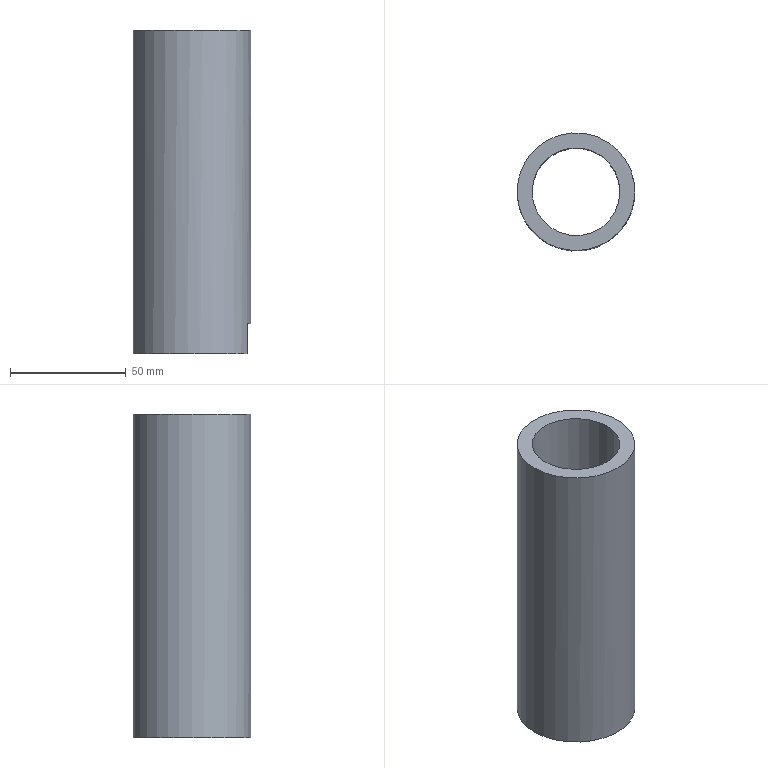Part | NX | features solid 2 | 1 solid | 7 faces | box 51 x 51 x 140 mm | volume 125652 mm3 | plane 5 | cylinder 2 | commonest cylinder face diameters 38 x1 51 x1
STEP:
#1=CARTESIAN_POINT('',(329.506,538.888,40.));
#2=VERTEX_POINT('',#1);
#3=CARTESIAN_POINT('',(348.506,538.888,40.));
#4=DIRECTION('',(0.,0.,1.));
#5=DIRECTION('',(-1.,0.,0.));
#6=AXIS2_PLACEMENT_3D('',#3,#4,#5);
#7=CIRCLE('',#6,19.);
#8=EDGE_CURVE('',#2,#2,#7,.F.);
#9=ORIENTED_EDGE('',*,*,#8,.T.);
#10=EDGE_LOOP('',(#9));
#11=FACE_BOUND('',#10,.T.);
#12=CARTESIAN_POINT('',(323.006,538.888,40.));
#13=VERTEX_POINT('',#12);
#14=CARTESIAN_POINT('',(348.506,538.888,40.));
#15=DIRECTION('',(0.,0.,1.));
#16=DIRECTION('',(-1.,0.,0.));
#17=AXIS2_PLACEMENT_3D('',#14,#15,#16);
#18=CIRCLE('',#17,25.5);
#19=EDGE_CURVE('',#13,#13,#18,.F.);
#20=ORIENTED_EDGE('',*,*,#19,.F.);
#21=EDGE_LOOP('',(#20));
#22=FACE_BOUND('',#21,.T.);
#23=CARTESIAN_POINT('',(348.506,538.888,40.));
#24=DIRECTION('',(0.,0.,1.));
#25=DIRECTION('',(1.,0.,0.));
#26=AXIS2_PLACEMENT_3D('',#23,#24,#25);
#27=PLANE('',#26);
#28=ADVANCED_FACE('',(#11,#22),#27,.T.);
#29=CARTESIAN_POINT('',(365.239,547.888,-100.));
#30=VERTEX_POINT('',#29);
#31=CARTESIAN_POINT('',(372.365,547.888,-100.));
#32=VERTEX_POINT('',#31);
#33=CARTESIAN_POINT('',(348.506,547.888,-100.));
#34=DIRECTION('',(1.,0.,0.));
#35=VECTOR('',#34,1000.);
#36=LINE('',#33,#35);
#37=EDGE_CURVE('',#30,#32,#36,.T.);
#38=ORIENTED_EDGE('',*,*,#37,.F.);
#39=CARTESIAN_POINT('',(365.239,529.888,-100.));
#40=VERTEX_POINT('',#39);
#41=CARTESIAN_POINT('',(348.506,538.888,-100.));
#42=DIRECTION('',(0.,0.,-1.));
#43=DIRECTION('',(0.,-1.,0.));
#44=AXIS2_PLACEMENT_3D('',#41,#42,#43);
#45=CIRCLE('',#44,19.);
#46=EDGE_CURVE('',#40,#30,#45,.T.);
#47=ORIENTED_EDGE('',*,*,#46,.F.);
#48=CARTESIAN_POINT('',(372.365,529.888,-100.));
#49=VERTEX_POINT('',#48);
#50=CARTESIAN_POINT('',(348.506,529.888,-100.));
#51=DIRECTION('',(1.,0.,0.));
#52=VECTOR('',#51,1000.);
#53=LINE('',#50,#52);
#54=EDGE_CURVE('',#40,#49,#53,.T.);
#55=ORIENTED_EDGE('',*,*,#54,.T.);
#56=CARTESIAN_POINT('',(348.506,538.888,-100.));
#57=DIRECTION('',(0.,0.,1.));
#58=DIRECTION('',(0.,1.,0.));
#59=AXIS2_PLACEMENT_3D('',#56,#57,#58);
#60=CIRCLE('',#59,25.5);
#61=EDGE_CURVE('',#32,#49,#60,.T.);
#62=ORIENTED_EDGE('',*,*,#61,.F.);
#63=EDGE_LOOP('',(#38,#47,#55,#62));
#64=FACE_BOUND('',#63,.T.);
#65=CARTESIAN_POINT('',(348.506,538.888,-100.));
#66=DIRECTION('',(0.,0.,-1.));
#67=DIRECTION('',(0.,-1.,0.));
#68=AXIS2_PLACEMENT_3D('',#65,#66,#67);
#69=PLANE('',#68);
#70=ADVANCED_FACE('',(#64),#69,.T.);
#71=CARTESIAN_POINT('',(372.365,547.888,-87.));
#72=VERTEX_POINT('',#71);
#73=CARTESIAN_POINT('',(372.365,547.888,-100.));
#74=DIRECTION('',(0.,0.,1.));
#75=VECTOR('',#74,1000.);
#76=LINE('',#73,#75);
#77=EDGE_CURVE('',#32,#72,#76,.T.);
#78=ORIENTED_EDGE('',*,*,#77,.F.);
#79=ORIENTED_EDGE('',*,*,#61,.T.);
#80=CARTESIAN_POINT('',(372.365,529.888,-87.));
#81=VERTEX_POINT('',#80);
#82=CARTESIAN_POINT('',(372.365,529.888,-100.));
#83=DIRECTION('',(0.,0.,1.));
#84=VECTOR('',#83,1000.);
#85=LINE('',#82,#84);
#86=EDGE_CURVE('',#49,#81,#85,.T.);
#87=ORIENTED_EDGE('',*,*,#86,.T.);
#88=CARTESIAN_POINT('',(348.506,538.888,-87.));
#89=DIRECTION('',(0.,0.,1.));
#90=DIRECTION('',(0.,1.,0.));
#91=AXIS2_PLACEMENT_3D('',#88,#89,#90);
#92=CIRCLE('',#91,25.5);
#93=EDGE_CURVE('',#72,#81,#92,.F.);
#94=ORIENTED_EDGE('',*,*,#93,.F.);
#95=EDGE_LOOP('',(#78,#79,#87,#94));
#96=FACE_BOUND('',#95,.T.);
#97=ORIENTED_EDGE('',*,*,#19,.T.);
#98=EDGE_LOOP('',(#97));
#99=FACE_BOUND('',#98,.T.);
#100=CARTESIAN_POINT('',(348.506,538.888,-100.));
#101=DIRECTION('',(0.,0.,1.));
#102=DIRECTION('',(0.,1.,0.));
#103=AXIS2_PLACEMENT_3D('',#100,#101,#102);
#104=CYLINDRICAL_SURFACE('',#103,25.5);
#105=ADVANCED_FACE('',(#96,#99),#104,.T.);
#106=ORIENTED_EDGE('',*,*,#46,.T.);
#107=CARTESIAN_POINT('',(365.239,547.888,-87.));
#108=VERTEX_POINT('',#107);
#109=CARTESIAN_POINT('',(365.239,547.888,-30.));
#110=DIRECTION('',(0.,0.,-1.));
#111=VECTOR('',#110,1000.);
#112=LINE('',#109,#111);
#113=EDGE_CURVE('',#30,#108,#112,.F.);
#114=ORIENTED_EDGE('',*,*,#113,.T.);
#115=CARTESIAN_POINT('',(365.239,529.888,-87.));
#116=VERTEX_POINT('',#115);
#117=CARTESIAN_POINT('',(348.506,538.888,-87.));
#118=DIRECTION('',(0.,0.,1.));
#119=DIRECTION('',(0.,1.,0.));
#120=AXIS2_PLACEMENT_3D('',#117,#118,#119);
#121=CIRCLE('',#120,19.);
#122=EDGE_CURVE('',#108,#116,#121,.F.);
#123=ORIENTED_EDGE('',*,*,#122,.T.);
#124=CARTESIAN_POINT('',(365.239,529.888,-30.));
#125=DIRECTION('',(0.,0.,-1.));
#126=VECTOR('',#125,1000.);
#127=LINE('',#124,#126);
#128=EDGE_CURVE('',#40,#116,#127,.F.);
#129=ORIENTED_EDGE('',*,*,#128,.F.);
#130=EDGE_LOOP('',(#106,#114,#123,#129));
#131=FACE_BOUND('',#130,.T.);
#132=ORIENTED_EDGE('',*,*,#8,.F.);
#133=EDGE_LOOP('',(#132));
#134=FACE_BOUND('',#133,.T.);
#135=CARTESIAN_POINT('',(348.506,538.888,-30.));
#136=DIRECTION('',(0.,0.,-1.));
#137=DIRECTION('',(0.,-1.,0.));
#138=AXIS2_PLACEMENT_3D('',#135,#136,#137);
#139=CYLINDRICAL_SURFACE('',#138,19.);
#140=ADVANCED_FACE('',(#131,#134),#139,.F.);
#141=ORIENTED_EDGE('',*,*,#93,.T.);
#142=CARTESIAN_POINT('',(428.506,529.888,-87.));
#143=DIRECTION('',(-1.,0.,0.));
#144=VECTOR('',#143,1000.);
#145=LINE('',#142,#144);
#146=EDGE_CURVE('',#81,#116,#145,.T.);
#147=ORIENTED_EDGE('',*,*,#146,.T.);
#148=ORIENTED_EDGE('',*,*,#122,.F.);
#149=CARTESIAN_POINT('',(428.506,547.888,-87.));
#150=DIRECTION('',(-1.,0.,0.));
#151=VECTOR('',#150,1000.);
#152=LINE('',#149,#151);
#153=EDGE_CURVE('',#72,#108,#152,.T.);
#154=ORIENTED_EDGE('',*,*,#153,.F.);
#155=EDGE_LOOP('',(#141,#147,#148,#154));
#156=FACE_BOUND('',#155,.T.);
#157=CARTESIAN_POINT('',(428.506,547.888,-87.));
#158=DIRECTION('',(0.,0.,1.));
#159=DIRECTION('',(0.,1.,0.));
#160=AXIS2_PLACEMENT_3D('',#157,#158,#159);
#161=PLANE('',#160);
#162=ADVANCED_FACE('',(#156),#161,.F.);
#163=ORIENTED_EDGE('',*,*,#77,.T.);
#164=ORIENTED_EDGE('',*,*,#153,.T.);
#165=ORIENTED_EDGE('',*,*,#113,.F.);
#166=ORIENTED_EDGE('',*,*,#37,.T.);
#167=EDGE_LOOP('',(#163,#164,#165,#166));
#168=FACE_BOUND('',#167,.T.);
#169=CARTESIAN_POINT('',(288.506,547.888,-80.));
#170=DIRECTION('',(0.,1.,0.));
#171=DIRECTION('',(0.,0.,1.));
#172=AXIS2_PLACEMENT_3D('',#169,#170,#171);
#173=PLANE('',#172);
#174=ADVANCED_FACE('',(#168),#173,.F.);
#175=ORIENTED_EDGE('',*,*,#54,.F.);
#176=ORIENTED_EDGE('',*,*,#128,.T.);
#177=ORIENTED_EDGE('',*,*,#146,.F.);
#178=ORIENTED_EDGE('',*,*,#86,.F.);
#179=EDGE_LOOP('',(#175,#176,#177,#178));
#180=FACE_BOUND('',#179,.T.);
#181=CARTESIAN_POINT('',(288.506,529.888,-80.));
#182=DIRECTION('',(0.,1.,0.));
#183=DIRECTION('',(0.,0.,1.));
#184=AXIS2_PLACEMENT_3D('',#181,#182,#183);
#185=PLANE('',#184);
#186=ADVANCED_FACE('',(#180),#185,.T.);
#187=CLOSED_SHELL('',(#28,#70,#105,#140,#162,#174,#186));
#188=MANIFOLD_SOLID_BREP('',#187);
#189=(LENGTH_UNIT()NAMED_UNIT(*)SI_UNIT(.MILLI.,.METRE.));
#190=UNCERTAINTY_MEASURE_WITH_UNIT(LENGTH_MEASURE(0.00001),#189,'','');
#191=(NAMED_UNIT(*)PLANE_ANGLE_UNIT()SI_UNIT($,.RADIAN.));
#192=(NAMED_UNIT(*)SI_UNIT($,.STERADIAN.)SOLID_ANGLE_UNIT());
#193=(GEOMETRIC_REPRESENTATION_CONTEXT(3)GLOBAL_UNCERTAINTY_ASSIGNED_CONTEXT((#190))GLOBAL_UNIT_ASSIGNED_CONTEXT((#189,#191,#192))REPRESENTATION_CONTEXT('',''));
#194=ADVANCED_BREP_SHAPE_REPRESENTATION('',(#188),#193);